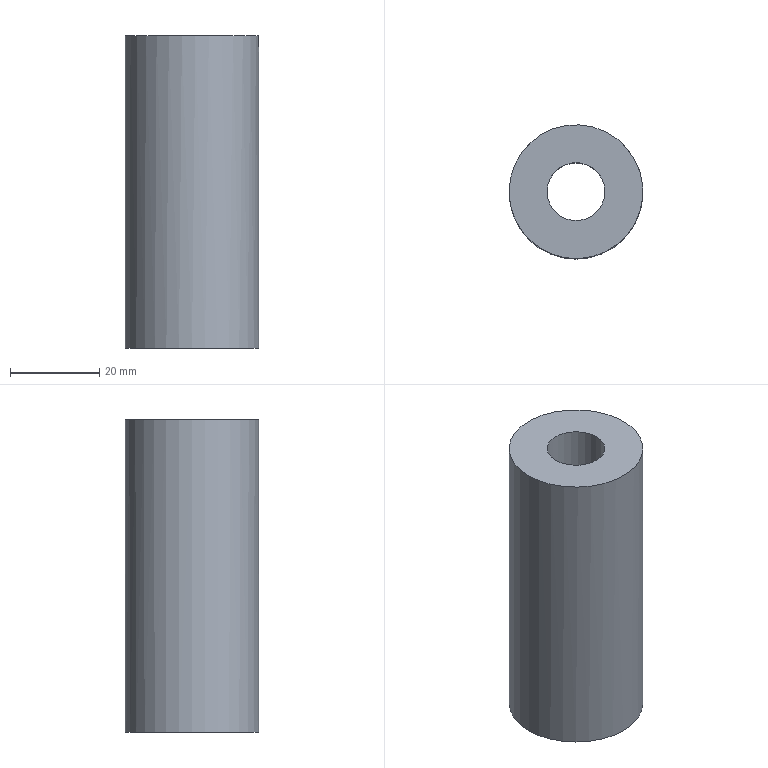Part | NX | features solid 2 | 1 solid | 6 faces | box 30 x 30 x 70 mm | volume 33839 mm3 | plane 3 | cylinder 3 | commonest cylinder face diameters 13 x1 20 x1 30 x1
STEP:
#1=CARTESIAN_POINT('',(373.5,-773.051,35.));
#2=VERTEX_POINT('',#1);
#3=CARTESIAN_POINT('',(380.,-773.051,35.));
#4=DIRECTION('',(-0.000000502,-0.000000149,-1.));
#5=DIRECTION('',(-1.,0.,0.000000502));
#6=AXIS2_PLACEMENT_3D('',#3,#4,#5);
#7=CIRCLE('',#6,6.5);
#8=EDGE_CURVE('',#2,#2,#7,.T.);
#9=ORIENTED_EDGE('',*,*,#8,.T.);
#10=EDGE_LOOP('',(#9));
#11=FACE_BOUND('',#10,.T.);
#12=CARTESIAN_POINT('',(365.,-773.051,35.));
#13=VERTEX_POINT('',#12);
#14=CARTESIAN_POINT('',(380.,-773.051,35.));
#15=DIRECTION('',(-0.000000502,-0.000000149,-1.));
#16=DIRECTION('',(-1.,0.,0.000000502));
#17=AXIS2_PLACEMENT_3D('',#14,#15,#16);
#18=CIRCLE('',#17,15.);
#19=EDGE_CURVE('',#13,#13,#18,.F.);
#20=ORIENTED_EDGE('',*,*,#19,.T.);
#21=EDGE_LOOP('',(#20));
#22=FACE_BOUND('',#21,.T.);
#23=CARTESIAN_POINT('',(380.,-773.051,35.));
#24=DIRECTION('',(0.000000502,0.000000149,1.));
#25=DIRECTION('',(-1.,0.000001668,0.000000502));
#26=AXIS2_PLACEMENT_3D('',#23,#24,#25);
#27=PLANE('',#26);
#28=ADVANCED_FACE('',(#11,#22),#27,.T.);
#29=CARTESIAN_POINT('',(370.,-773.051,-35.));
#30=VERTEX_POINT('',#29);
#31=CARTESIAN_POINT('',(380.,-773.051,-35.));
#32=DIRECTION('',(-0.000000502,-0.000000149,-1.));
#33=DIRECTION('',(-1.,0.000001668,0.000000502));
#34=AXIS2_PLACEMENT_3D('',#31,#32,#33);
#35=CIRCLE('',#34,10.);
#36=EDGE_CURVE('',#30,#30,#35,.T.);
#37=ORIENTED_EDGE('',*,*,#36,.F.);
#38=EDGE_LOOP('',(#37));
#39=FACE_BOUND('',#38,.T.);
#40=CARTESIAN_POINT('',(395.,-773.051,-35.));
#41=VERTEX_POINT('',#40);
#42=CARTESIAN_POINT('',(380.,-773.051,-35.));
#43=DIRECTION('',(0.000000502,0.000000149,1.));
#44=DIRECTION('',(1.,-0.000001668,-0.000000502));
#45=AXIS2_PLACEMENT_3D('',#42,#43,#44);
#46=CIRCLE('',#45,15.);
#47=EDGE_CURVE('',#41,#41,#46,.F.);
#48=ORIENTED_EDGE('',*,*,#47,.T.);
#49=EDGE_LOOP('',(#48));
#50=FACE_BOUND('',#49,.T.);
#51=CARTESIAN_POINT('',(380.,-773.051,-35.));
#52=DIRECTION('',(-0.000000502,-0.000000149,-1.));
#53=DIRECTION('',(1.,-0.000001668,-0.000000502));
#54=AXIS2_PLACEMENT_3D('',#51,#52,#53);
#55=PLANE('',#54);
#56=ADVANCED_FACE('',(#39,#50),#55,.T.);
#57=ORIENTED_EDGE('',*,*,#19,.F.);
#58=EDGE_LOOP('',(#57));
#59=FACE_BOUND('',#58,.T.);
#60=ORIENTED_EDGE('',*,*,#47,.F.);
#61=EDGE_LOOP('',(#60));
#62=FACE_BOUND('',#61,.T.);
#63=CARTESIAN_POINT('',(380.,-773.051,-50.));
#64=DIRECTION('',(0.000000502,0.000000149,1.));
#65=DIRECTION('',(-1.,0.000001668,0.000000502));
#66=AXIS2_PLACEMENT_3D('',#63,#64,#65);
#67=CYLINDRICAL_SURFACE('',#66,15.);
#68=ADVANCED_FACE('',(#59,#62),#67,.T.);
#69=ORIENTED_EDGE('',*,*,#8,.F.);
#70=EDGE_LOOP('',(#69));
#71=FACE_BOUND('',#70,.T.);
#72=CARTESIAN_POINT('',(373.5,-773.051,-0.00001086));
#73=VERTEX_POINT('',#72);
#74=CARTESIAN_POINT('',(380.,-773.051,-0.00001412));
#75=DIRECTION('',(-0.000000502,-0.000000149,-1.));
#76=DIRECTION('',(-1.,0.000001668,0.000000502));
#77=AXIS2_PLACEMENT_3D('',#74,#75,#76);
#78=CIRCLE('',#77,6.5);
#79=EDGE_CURVE('',#73,#73,#78,.T.);
#80=ORIENTED_EDGE('',*,*,#79,.T.);
#81=EDGE_LOOP('',(#80));
#82=FACE_BOUND('',#81,.T.);
#83=CARTESIAN_POINT('',(380.,-773.051,65.));
#84=DIRECTION('',(0.000000502,0.000000149,1.));
#85=DIRECTION('',(-1.,0.000001668,0.000000502));
#86=AXIS2_PLACEMENT_3D('',#83,#84,#85);
#87=CYLINDRICAL_SURFACE('',#86,6.5);
#88=ADVANCED_FACE('',(#71,#82),#87,.F.);
#89=ORIENTED_EDGE('',*,*,#79,.F.);
#90=EDGE_LOOP('',(#89));
#91=FACE_BOUND('',#90,.T.);
#92=CARTESIAN_POINT('',(370.,-773.051,-0.0000091));
#93=VERTEX_POINT('',#92);
#94=CARTESIAN_POINT('',(380.,-773.051,-0.00001412));
#95=DIRECTION('',(-0.000000502,-0.000000149,-1.));
#96=DIRECTION('',(-1.,0.000001668,0.000000502));
#97=AXIS2_PLACEMENT_3D('',#94,#95,#96);
#98=CIRCLE('',#97,10.);
#99=EDGE_CURVE('',#93,#93,#98,.T.);
#100=ORIENTED_EDGE('',*,*,#99,.T.);
#101=EDGE_LOOP('',(#100));
#102=FACE_BOUND('',#101,.T.);
#103=CARTESIAN_POINT('',(380.,-773.051,-0.00001412));
#104=DIRECTION('',(0.000000502,0.000000149,1.));
#105=DIRECTION('',(-1.,0.000001668,0.000000502));
#106=AXIS2_PLACEMENT_3D('',#103,#104,#105);
#107=PLANE('',#106);
#108=ADVANCED_FACE('',(#91,#102),#107,.F.);
#109=ORIENTED_EDGE('',*,*,#99,.F.);
#110=EDGE_LOOP('',(#109));
#111=FACE_BOUND('',#110,.T.);
#112=ORIENTED_EDGE('',*,*,#36,.T.);
#113=EDGE_LOOP('',(#112));
#114=FACE_BOUND('',#113,.T.);
#115=CARTESIAN_POINT('',(380.,-773.051,-35.));
#116=DIRECTION('',(0.000000502,0.000000149,1.));
#117=DIRECTION('',(-1.,0.000001668,0.000000502));
#118=AXIS2_PLACEMENT_3D('',#115,#116,#117);
#119=CYLINDRICAL_SURFACE('',#118,10.);
#120=ADVANCED_FACE('',(#111,#114),#119,.F.);
#121=CLOSED_SHELL('',(#28,#56,#68,#88,#108,#120));
#122=MANIFOLD_SOLID_BREP('',#121);
#123=(LENGTH_UNIT()NAMED_UNIT(*)SI_UNIT(.MILLI.,.METRE.));
#124=UNCERTAINTY_MEASURE_WITH_UNIT(LENGTH_MEASURE(0.00001),#123,'','');
#125=(NAMED_UNIT(*)PLANE_ANGLE_UNIT()SI_UNIT($,.RADIAN.));
#126=(NAMED_UNIT(*)SI_UNIT($,.STERADIAN.)SOLID_ANGLE_UNIT());
#127=(GEOMETRIC_REPRESENTATION_CONTEXT(3)GLOBAL_UNCERTAINTY_ASSIGNED_CONTEXT((#124))GLOBAL_UNIT_ASSIGNED_CONTEXT((#123,#125,#126))REPRESENTATION_CONTEXT('',''));
#128=ADVANCED_BREP_SHAPE_REPRESENTATION('',(#122),#127);